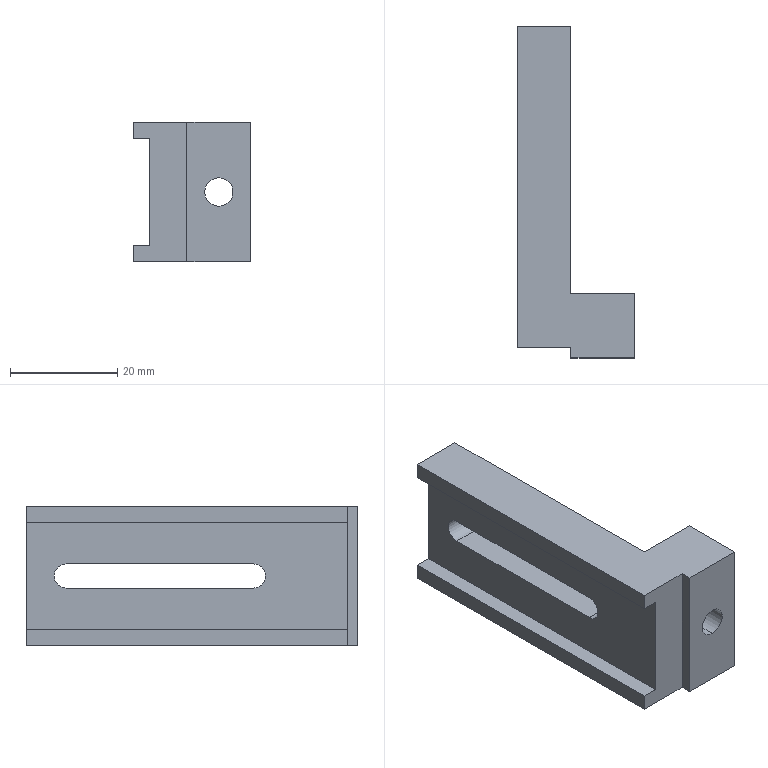Part | NX | features BREP 1 | 1 solid | 23 faces | box 21.97 x 62 x 26 mm | volume 13950 mm3 | plane 17 | cylinder 6 | commonest cylinder face diameters 4.5 x2 5.3 x2 10 x2
STEP:
#1=CARTESIAN_POINT('',(6.,-5.4,7.));
#2=VERTEX_POINT('',#1);
#3=CARTESIAN_POINT('',(6.,-5.4,17.));
#4=VERTEX_POINT('',#3);
#5=CARTESIAN_POINT('',(6.,-5.4,12.));
#6=DIRECTION('',(0.,1.,0.));
#7=DIRECTION('',(0.,0.,1.));
#8=AXIS2_PLACEMENT_3D('',#5,#6,#7);
#9=CIRCLE('',#8,5.);
#10=EDGE_CURVE('',#2,#4,#9,.T.);
#11=ORIENTED_EDGE('',*,*,#10,.F.);
#12=CARTESIAN_POINT('',(6.,0.,7.));
#13=VERTEX_POINT('',#12);
#14=CARTESIAN_POINT('',(6.,0.,7.));
#15=DIRECTION('',(0.,1.,0.));
#16=VECTOR('',#15,1000.);
#17=LINE('',#14,#16);
#18=EDGE_CURVE('',#13,#2,#17,.F.);
#19=ORIENTED_EDGE('',*,*,#18,.F.);
#20=CARTESIAN_POINT('',(6.,0.,17.));
#21=VERTEX_POINT('',#20);
#22=CARTESIAN_POINT('',(6.,0.,12.));
#23=DIRECTION('',(0.,1.,0.));
#24=DIRECTION('',(0.,0.,1.));
#25=AXIS2_PLACEMENT_3D('',#22,#23,#24);
#26=CIRCLE('',#25,5.);
#27=EDGE_CURVE('',#13,#21,#26,.T.);
#28=ORIENTED_EDGE('',*,*,#27,.T.);
#29=CARTESIAN_POINT('',(6.,0.,17.));
#30=DIRECTION('',(0.,1.,0.));
#31=VECTOR('',#30,1000.);
#32=LINE('',#29,#31);
#33=EDGE_CURVE('',#21,#4,#32,.F.);
#34=ORIENTED_EDGE('',*,*,#33,.T.);
#35=EDGE_LOOP('',(#11,#19,#28,#34));
#36=FACE_BOUND('',#35,.T.);
#37=CARTESIAN_POINT('',(6.,0.,12.));
#38=DIRECTION('',(0.,1.,0.));
#39=DIRECTION('',(0.,0.,1.));
#40=AXIS2_PLACEMENT_3D('',#37,#38,#39);
#41=CYLINDRICAL_SURFACE('',#40,5.);
#42=ADVANCED_FACE('',(#36),#41,.F.);
#43=CARTESIAN_POINT('',(6.,-12.,9.35));
#44=VERTEX_POINT('',#43);
#45=CARTESIAN_POINT('',(6.,-12.,14.65));
#46=VERTEX_POINT('',#45);
#47=CARTESIAN_POINT('',(6.,-12.,12.));
#48=DIRECTION('',(0.,1.,0.));
#49=DIRECTION('',(0.,0.,1.));
#50=AXIS2_PLACEMENT_3D('',#47,#48,#49);
#51=CIRCLE('',#50,2.65);
#52=EDGE_CURVE('',#44,#46,#51,.T.);
#53=ORIENTED_EDGE('',*,*,#52,.F.);
#54=CARTESIAN_POINT('',(6.,-5.4,9.35));
#55=VERTEX_POINT('',#54);
#56=CARTESIAN_POINT('',(6.,0.,9.35));
#57=DIRECTION('',(0.,1.,0.));
#58=VECTOR('',#57,1000.);
#59=LINE('',#56,#58);
#60=EDGE_CURVE('',#55,#44,#59,.F.);
#61=ORIENTED_EDGE('',*,*,#60,.F.);
#62=CARTESIAN_POINT('',(6.,-5.4,14.65));
#63=VERTEX_POINT('',#62);
#64=CARTESIAN_POINT('',(6.,-5.4,12.));
#65=DIRECTION('',(0.,1.,0.));
#66=DIRECTION('',(0.,0.,1.));
#67=AXIS2_PLACEMENT_3D('',#64,#65,#66);
#68=CIRCLE('',#67,2.65);
#69=EDGE_CURVE('',#55,#63,#68,.T.);
#70=ORIENTED_EDGE('',*,*,#69,.T.);
#71=CARTESIAN_POINT('',(6.,0.,14.65));
#72=DIRECTION('',(0.,1.,0.));
#73=VECTOR('',#72,1000.);
#74=LINE('',#71,#73);
#75=EDGE_CURVE('',#63,#46,#74,.F.);
#76=ORIENTED_EDGE('',*,*,#75,.T.);
#77=EDGE_LOOP('',(#53,#61,#70,#76));
#78=FACE_BOUND('',#77,.T.);
#79=CARTESIAN_POINT('',(6.,0.,12.));
#80=DIRECTION('',(0.,1.,0.));
#81=DIRECTION('',(0.,0.,1.));
#82=AXIS2_PLACEMENT_3D('',#79,#80,#81);
#83=CYLINDRICAL_SURFACE('',#82,2.65);
#84=ADVANCED_FACE('',(#78),#83,.F.);
#85=CARTESIAN_POINT('',(-10.,50.,25.));
#86=VERTEX_POINT('',#85);
#87=CARTESIAN_POINT('',(-10.,50.,22.));
#88=VERTEX_POINT('',#87);
#89=CARTESIAN_POINT('',(-10.,50.,24.));
#90=DIRECTION('',(0.,0.,-1.));
#91=VECTOR('',#90,1000.);
#92=LINE('',#89,#91);
#93=EDGE_CURVE('',#86,#88,#92,.T.);
#94=ORIENTED_EDGE('',*,*,#93,.T.);
#95=CARTESIAN_POINT('',(-10.,-10.,22.));
#96=VERTEX_POINT('',#95);
#97=CARTESIAN_POINT('',(-10.,0.,22.));
#98=DIRECTION('',(0.,-1.,0.));
#99=VECTOR('',#98,1000.);
#100=LINE('',#97,#99);
#101=EDGE_CURVE('',#88,#96,#100,.T.);
#102=ORIENTED_EDGE('',*,*,#101,.T.);
#103=CARTESIAN_POINT('',(-10.,-10.,25.));
#104=VERTEX_POINT('',#103);
#105=CARTESIAN_POINT('',(-10.,-10.,24.));
#106=DIRECTION('',(0.,0.,-1.));
#107=VECTOR('',#106,1000.);
#108=LINE('',#105,#107);
#109=EDGE_CURVE('',#104,#96,#108,.T.);
#110=ORIENTED_EDGE('',*,*,#109,.F.);
#111=CARTESIAN_POINT('',(-10.,0.,25.));
#112=DIRECTION('',(0.,-1.,0.));
#113=VECTOR('',#112,1000.);
#114=LINE('',#111,#113);
#115=EDGE_CURVE('',#86,#104,#114,.T.);
#116=ORIENTED_EDGE('',*,*,#115,.F.);
#117=EDGE_LOOP('',(#94,#102,#110,#116));
#118=FACE_BOUND('',#117,.T.);
#119=CARTESIAN_POINT('',(-10.,0.,24.));
#120=DIRECTION('',(1.,0.,0.));
#121=DIRECTION('',(0.,1.,0.));
#122=AXIS2_PLACEMENT_3D('',#119,#120,#121);
#123=PLANE('',#122);
#124=ADVANCED_FACE('',(#118),#123,.F.);
#125=ORIENTED_EDGE('',*,*,#109,.T.);
#126=CARTESIAN_POINT('',(-7.,-10.,22.));
#127=VERTEX_POINT('',#126);
#128=CARTESIAN_POINT('',(0.,-10.,22.));
#129=DIRECTION('',(1.,0.,0.));
#130=VECTOR('',#129,1000.);
#131=LINE('',#128,#130);
#132=EDGE_CURVE('',#96,#127,#131,.T.);
#133=ORIENTED_EDGE('',*,*,#132,.T.);
#134=CARTESIAN_POINT('',(-7.,-10.,2.));
#135=VERTEX_POINT('',#134);
#136=CARTESIAN_POINT('',(-7.,-10.,24.));
#137=DIRECTION('',(0.,0.,1.));
#138=VECTOR('',#137,1000.);
#139=LINE('',#136,#138);
#140=EDGE_CURVE('',#135,#127,#139,.T.);
#141=ORIENTED_EDGE('',*,*,#140,.F.);
#142=CARTESIAN_POINT('',(-10.,-10.,2.));
#143=VERTEX_POINT('',#142);
#144=CARTESIAN_POINT('',(0.,-10.,2.));
#145=DIRECTION('',(-1.,0.,0.));
#146=VECTOR('',#145,1000.);
#147=LINE('',#144,#146);
#148=EDGE_CURVE('',#135,#143,#147,.T.);
#149=ORIENTED_EDGE('',*,*,#148,.T.);
#150=CARTESIAN_POINT('',(-10.,-10.,-1.));
#151=VERTEX_POINT('',#150);
#152=CARTESIAN_POINT('',(-10.,-10.,24.));
#153=DIRECTION('',(0.,0.,-1.));
#154=VECTOR('',#153,1000.);
#155=LINE('',#152,#154);
#156=EDGE_CURVE('',#143,#151,#155,.T.);
#157=ORIENTED_EDGE('',*,*,#156,.T.);
#158=CARTESIAN_POINT('',(0.03,-10.,-1.));
#159=VERTEX_POINT('',#158);
#160=CARTESIAN_POINT('',(0.,-10.,-1.));
#161=DIRECTION('',(1.,0.,0.));
#162=VECTOR('',#161,1000.);
#163=LINE('',#160,#162);
#164=EDGE_CURVE('',#151,#159,#163,.T.);
#165=ORIENTED_EDGE('',*,*,#164,.T.);
#166=CARTESIAN_POINT('',(0.03,-10.,25.));
#167=VERTEX_POINT('',#166);
#168=CARTESIAN_POINT('',(0.03,-10.,0.));
#169=DIRECTION('',(0.,0.,-1.));
#170=VECTOR('',#169,1000.);
#171=LINE('',#168,#170);
#172=EDGE_CURVE('',#167,#159,#171,.T.);
#173=ORIENTED_EDGE('',*,*,#172,.F.);
#174=CARTESIAN_POINT('',(0.,-10.,25.));
#175=DIRECTION('',(1.,0.,0.));
#176=VECTOR('',#175,1000.);
#177=LINE('',#174,#176);
#178=EDGE_CURVE('',#104,#167,#177,.T.);
#179=ORIENTED_EDGE('',*,*,#178,.F.);
#180=EDGE_LOOP('',(#125,#133,#141,#149,#157,#165,#173,#179));
#181=FACE_BOUND('',#180,.T.);
#182=CARTESIAN_POINT('',(0.,-10.,24.));
#183=DIRECTION('',(0.,1.,0.));
#184=DIRECTION('',(1.,0.,0.));
#185=AXIS2_PLACEMENT_3D('',#182,#183,#184);
#186=PLANE('',#185);
#187=ADVANCED_FACE('',(#181),#186,.F.);
#188=CARTESIAN_POINT('',(11.97,0.,-1.));
#189=VERTEX_POINT('',#188);
#190=CARTESIAN_POINT('',(11.97,-12.,-1.));
#191=VERTEX_POINT('',#190);
#192=CARTESIAN_POINT('',(11.97,0.,-1.));
#193=DIRECTION('',(0.,-1.,0.));
#194=VECTOR('',#193,1000.);
#195=LINE('',#192,#194);
#196=EDGE_CURVE('',#189,#191,#195,.T.);
#197=ORIENTED_EDGE('',*,*,#196,.F.);
#198=CARTESIAN_POINT('',(11.97,0.,25.));
#199=VERTEX_POINT('',#198);
#200=CARTESIAN_POINT('',(11.97,0.,24.));
#201=DIRECTION('',(0.,0.,-1.));
#202=VECTOR('',#201,1000.);
#203=LINE('',#200,#202);
#204=EDGE_CURVE('',#199,#189,#203,.T.);
#205=ORIENTED_EDGE('',*,*,#204,.F.);
#206=CARTESIAN_POINT('',(11.97,-12.,25.));
#207=VERTEX_POINT('',#206);
#208=CARTESIAN_POINT('',(11.97,0.,25.));
#209=DIRECTION('',(0.,-1.,0.));
#210=VECTOR('',#209,1000.);
#211=LINE('',#208,#210);
#212=EDGE_CURVE('',#199,#207,#211,.T.);
#213=ORIENTED_EDGE('',*,*,#212,.T.);
#214=CARTESIAN_POINT('',(11.97,-12.,0.));
#215=DIRECTION('',(0.,0.,1.));
#216=VECTOR('',#215,1000.);
#217=LINE('',#214,#216);
#218=EDGE_CURVE('',#191,#207,#217,.T.);
#219=ORIENTED_EDGE('',*,*,#218,.F.);
#220=EDGE_LOOP('',(#197,#205,#213,#219));
#221=FACE_BOUND('',#220,.T.);
#222=CARTESIAN_POINT('',(11.97,0.,24.));
#223=DIRECTION('',(1.,0.,0.));
#224=DIRECTION('',(0.,1.,0.));
#225=AXIS2_PLACEMENT_3D('',#222,#223,#224);
#226=PLANE('',#225);
#227=ADVANCED_FACE('',(#221),#226,.T.);
#228=CARTESIAN_POINT('',(0.,0.,-1.));
#229=VERTEX_POINT('',#228);
#230=CARTESIAN_POINT('',(0.,0.,-1.));
#231=DIRECTION('',(1.,0.,0.));
#232=VECTOR('',#231,1000.);
#233=LINE('',#230,#232);
#234=EDGE_CURVE('',#229,#189,#233,.T.);
#235=ORIENTED_EDGE('',*,*,#234,.F.);
#236=CARTESIAN_POINT('',(0.,0.,25.));
#237=VERTEX_POINT('',#236);
#238=CARTESIAN_POINT('',(0.,0.,24.));
#239=DIRECTION('',(0.,0.,-1.));
#240=VECTOR('',#239,1000.);
#241=LINE('',#238,#240);
#242=EDGE_CURVE('',#237,#229,#241,.T.);
#243=ORIENTED_EDGE('',*,*,#242,.F.);
#244=CARTESIAN_POINT('',(0.,0.,25.));
#245=DIRECTION('',(1.,0.,0.));
#246=VECTOR('',#245,1000.);
#247=LINE('',#244,#246);
#248=EDGE_CURVE('',#237,#199,#247,.T.);
#249=ORIENTED_EDGE('',*,*,#248,.T.);
#250=ORIENTED_EDGE('',*,*,#204,.T.);
#251=EDGE_LOOP('',(#235,#243,#249,#250));
#252=FACE_BOUND('',#251,.T.);
#253=CARTESIAN_POINT('',(6.,0.,12.));
#254=DIRECTION('',(0.,1.,0.));
#255=DIRECTION('',(0.,0.,1.));
#256=AXIS2_PLACEMENT_3D('',#253,#254,#255);
#257=CIRCLE('',#256,5.);
#258=EDGE_CURVE('',#21,#13,#257,.T.);
#259=ORIENTED_EDGE('',*,*,#258,.F.);
#260=ORIENTED_EDGE('',*,*,#27,.F.);
#261=EDGE_LOOP('',(#259,#260));
#262=FACE_BOUND('',#261,.T.);
#263=CARTESIAN_POINT('',(0.,0.,24.));
#264=DIRECTION('',(0.,1.,0.));
#265=DIRECTION('',(1.,0.,0.));
#266=AXIS2_PLACEMENT_3D('',#263,#264,#265);
#267=PLANE('',#266);
#268=ADVANCED_FACE('',(#252,#262),#267,.T.);
#269=CARTESIAN_POINT('',(0.,50.,-1.));
#270=VERTEX_POINT('',#269);
#271=CARTESIAN_POINT('',(0.,0.,-1.));
#272=DIRECTION('',(0.,-1.,0.));
#273=VECTOR('',#272,1000.);
#274=LINE('',#271,#273);
#275=EDGE_CURVE('',#270,#229,#274,.T.);
#276=ORIENTED_EDGE('',*,*,#275,.F.);
#277=CARTESIAN_POINT('',(0.,50.,25.));
#278=VERTEX_POINT('',#277);
#279=CARTESIAN_POINT('',(0.,50.,24.));
#280=DIRECTION('',(0.,0.,-1.));
#281=VECTOR('',#280,1000.);
#282=LINE('',#279,#281);
#283=EDGE_CURVE('',#278,#270,#282,.T.);
#284=ORIENTED_EDGE('',*,*,#283,.F.);
#285=CARTESIAN_POINT('',(0.,0.,25.));
#286=DIRECTION('',(0.,-1.,0.));
#287=VECTOR('',#286,1000.);
#288=LINE('',#285,#287);
#289=EDGE_CURVE('',#278,#237,#288,.T.);
#290=ORIENTED_EDGE('',*,*,#289,.T.);
#291=ORIENTED_EDGE('',*,*,#242,.T.);
#292=EDGE_LOOP('',(#276,#284,#290,#291));
#293=FACE_BOUND('',#292,.T.);
#294=CARTESIAN_POINT('',(0.,7.5,14.25));
#295=VERTEX_POINT('',#294);
#296=CARTESIAN_POINT('',(0.,7.5,9.75));
#297=VERTEX_POINT('',#296);
#298=CARTESIAN_POINT('',(0.,7.5,12.));
#299=DIRECTION('',(1.,0.,0.));
#300=DIRECTION('',(0.,0.,-1.));
#301=AXIS2_PLACEMENT_3D('',#298,#299,#300);
#302=CIRCLE('',#301,2.25);
#303=EDGE_CURVE('',#295,#297,#302,.T.);
#304=ORIENTED_EDGE('',*,*,#303,.F.);
#305=CARTESIAN_POINT('',(0.,42.5,14.25));
#306=VERTEX_POINT('',#305);
#307=CARTESIAN_POINT('',(0.,7.5,14.25));
#308=DIRECTION('',(0.,-1.,0.));
#309=VECTOR('',#308,1000.);
#310=LINE('',#307,#309);
#311=EDGE_CURVE('',#306,#295,#310,.T.);
#312=ORIENTED_EDGE('',*,*,#311,.F.);
#313=CARTESIAN_POINT('',(0.,42.5,9.75));
#314=VERTEX_POINT('',#313);
#315=CARTESIAN_POINT('',(0.,42.5,12.));
#316=DIRECTION('',(1.,0.,0.));
#317=DIRECTION('',(0.,0.,-1.));
#318=AXIS2_PLACEMENT_3D('',#315,#316,#317);
#319=CIRCLE('',#318,2.25);
#320=EDGE_CURVE('',#314,#306,#319,.T.);
#321=ORIENTED_EDGE('',*,*,#320,.F.);
#322=CARTESIAN_POINT('',(0.,7.5,9.75));
#323=DIRECTION('',(0.,1.,0.));
#324=VECTOR('',#323,1000.);
#325=LINE('',#322,#324);
#326=EDGE_CURVE('',#297,#314,#325,.T.);
#327=ORIENTED_EDGE('',*,*,#326,.F.);
#328=EDGE_LOOP('',(#304,#312,#321,#327));
#329=FACE_BOUND('',#328,.T.);
#330=CARTESIAN_POINT('',(0.,0.,24.));
#331=DIRECTION('',(1.,0.,0.));
#332=DIRECTION('',(0.,1.,0.));
#333=AXIS2_PLACEMENT_3D('',#330,#331,#332);
#334=PLANE('',#333);
#335=ADVANCED_FACE('',(#293,#329),#334,.T.);
#336=CARTESIAN_POINT('',(-7.,50.,22.));
#337=VERTEX_POINT('',#336);
#338=CARTESIAN_POINT('',(-10.,50.,22.));
#339=DIRECTION('',(1.,0.,0.));
#340=VECTOR('',#339,1000.);
#341=LINE('',#338,#340);
#342=EDGE_CURVE('',#88,#337,#341,.T.);
#343=ORIENTED_EDGE('',*,*,#342,.F.);
#344=ORIENTED_EDGE('',*,*,#93,.F.);
#345=CARTESIAN_POINT('',(-10.,50.,25.));
#346=DIRECTION('',(1.,0.,0.));
#347=VECTOR('',#346,1000.);
#348=LINE('',#345,#347);
#349=EDGE_CURVE('',#86,#278,#348,.T.);
#350=ORIENTED_EDGE('',*,*,#349,.T.);
#351=ORIENTED_EDGE('',*,*,#283,.T.);
#352=CARTESIAN_POINT('',(-10.,50.,-1.));
#353=VERTEX_POINT('',#352);
#354=CARTESIAN_POINT('',(-10.,50.,-1.));
#355=DIRECTION('',(1.,0.,0.));
#356=VECTOR('',#355,1000.);
#357=LINE('',#354,#356);
#358=EDGE_CURVE('',#353,#270,#357,.T.);
#359=ORIENTED_EDGE('',*,*,#358,.F.);
#360=CARTESIAN_POINT('',(-10.,50.,2.));
#361=VERTEX_POINT('',#360);
#362=CARTESIAN_POINT('',(-10.,50.,24.));
#363=DIRECTION('',(0.,0.,-1.));
#364=VECTOR('',#363,1000.);
#365=LINE('',#362,#364);
#366=EDGE_CURVE('',#361,#353,#365,.T.);
#367=ORIENTED_EDGE('',*,*,#366,.F.);
#368=CARTESIAN_POINT('',(-7.,50.,2.));
#369=VERTEX_POINT('',#368);
#370=CARTESIAN_POINT('',(-10.,50.,2.));
#371=DIRECTION('',(-1.,0.,0.));
#372=VECTOR('',#371,1000.);
#373=LINE('',#370,#372);
#374=EDGE_CURVE('',#369,#361,#373,.T.);
#375=ORIENTED_EDGE('',*,*,#374,.F.);
#376=CARTESIAN_POINT('',(-7.,50.,24.));
#377=DIRECTION('',(0.,0.,1.));
#378=VECTOR('',#377,1000.);
#379=LINE('',#376,#378);
#380=EDGE_CURVE('',#369,#337,#379,.T.);
#381=ORIENTED_EDGE('',*,*,#380,.T.);
#382=EDGE_LOOP('',(#343,#344,#350,#351,#359,#367,#375,#381));
#383=FACE_BOUND('',#382,.T.);
#384=CARTESIAN_POINT('',(-10.,50.,24.));
#385=DIRECTION('',(0.,1.,0.));
#386=DIRECTION('',(1.,0.,0.));
#387=AXIS2_PLACEMENT_3D('',#384,#385,#386);
#388=PLANE('',#387);
#389=ADVANCED_FACE('',(#383),#388,.T.);
#390=ORIENTED_EDGE('',*,*,#156,.F.);
#391=CARTESIAN_POINT('',(-10.,0.,2.));
#392=DIRECTION('',(0.,1.,0.));
#393=VECTOR('',#392,1000.);
#394=LINE('',#391,#393);
#395=EDGE_CURVE('',#143,#361,#394,.T.);
#396=ORIENTED_EDGE('',*,*,#395,.T.);
#397=ORIENTED_EDGE('',*,*,#366,.T.);
#398=CARTESIAN_POINT('',(-10.,0.,-1.));
#399=DIRECTION('',(0.,-1.,0.));
#400=VECTOR('',#399,1000.);
#401=LINE('',#398,#400);
#402=EDGE_CURVE('',#353,#151,#401,.T.);
#403=ORIENTED_EDGE('',*,*,#402,.T.);
#404=EDGE_LOOP('',(#390,#396,#397,#403));
#405=FACE_BOUND('',#404,.T.);
#406=CARTESIAN_POINT('',(-10.,0.,24.));
#407=DIRECTION('',(1.,0.,0.));
#408=DIRECTION('',(0.,1.,0.));
#409=AXIS2_PLACEMENT_3D('',#406,#407,#408);
#410=PLANE('',#409);
#411=ADVANCED_FACE('',(#405),#410,.F.);
#412=ORIENTED_EDGE('',*,*,#178,.T.);
#413=CARTESIAN_POINT('',(0.03,-12.,25.));
#414=VERTEX_POINT('',#413);
#415=CARTESIAN_POINT('',(0.03,-12.,25.));
#416=DIRECTION('',(0.,1.,0.));
#417=VECTOR('',#416,1000.);
#418=LINE('',#415,#417);
#419=EDGE_CURVE('',#414,#167,#418,.T.);
#420=ORIENTED_EDGE('',*,*,#419,.F.);
#421=CARTESIAN_POINT('',(0.,-12.,25.));
#422=DIRECTION('',(-1.,0.,0.));
#423=VECTOR('',#422,1000.);
#424=LINE('',#421,#423);
#425=EDGE_CURVE('',#207,#414,#424,.T.);
#426=ORIENTED_EDGE('',*,*,#425,.F.);
#427=ORIENTED_EDGE('',*,*,#212,.F.);
#428=ORIENTED_EDGE('',*,*,#248,.F.);
#429=ORIENTED_EDGE('',*,*,#289,.F.);
#430=ORIENTED_EDGE('',*,*,#349,.F.);
#431=ORIENTED_EDGE('',*,*,#115,.T.);
#432=EDGE_LOOP('',(#412,#420,#426,#427,#428,#429,#430,#431));
#433=FACE_BOUND('',#432,.T.);
#434=CARTESIAN_POINT('',(0.,0.,25.));
#435=DIRECTION('',(0.,0.,-1.));
#436=DIRECTION('',(0.,-1.,0.));
#437=AXIS2_PLACEMENT_3D('',#434,#435,#436);
#438=PLANE('',#437);
#439=ADVANCED_FACE('',(#433),#438,.F.);
#440=ORIENTED_EDGE('',*,*,#164,.F.);
#441=ORIENTED_EDGE('',*,*,#402,.F.);
#442=ORIENTED_EDGE('',*,*,#358,.T.);
#443=ORIENTED_EDGE('',*,*,#275,.T.);
#444=ORIENTED_EDGE('',*,*,#234,.T.);
#445=ORIENTED_EDGE('',*,*,#196,.T.);
#446=CARTESIAN_POINT('',(0.03,-12.,-1.));
#447=VERTEX_POINT('',#446);
#448=CARTESIAN_POINT('',(0.,-12.,-1.));
#449=DIRECTION('',(1.,0.,0.));
#450=VECTOR('',#449,1000.);
#451=LINE('',#448,#450);
#452=EDGE_CURVE('',#447,#191,#451,.T.);
#453=ORIENTED_EDGE('',*,*,#452,.F.);
#454=CARTESIAN_POINT('',(0.03,-12.,-1.));
#455=DIRECTION('',(0.,1.,0.));
#456=VECTOR('',#455,1000.);
#457=LINE('',#454,#456);
#458=EDGE_CURVE('',#447,#159,#457,.T.);
#459=ORIENTED_EDGE('',*,*,#458,.T.);
#460=EDGE_LOOP('',(#440,#441,#442,#443,#444,#445,#453,#459));
#461=FACE_BOUND('',#460,.T.);
#462=CARTESIAN_POINT('',(0.,0.,-1.));
#463=DIRECTION('',(0.,0.,-1.));
#464=DIRECTION('',(0.,-1.,0.));
#465=AXIS2_PLACEMENT_3D('',#462,#463,#464);
#466=PLANE('',#465);
#467=ADVANCED_FACE('',(#461),#466,.T.);
#468=ORIENTED_EDGE('',*,*,#172,.T.);
#469=ORIENTED_EDGE('',*,*,#458,.F.);
#470=CARTESIAN_POINT('',(0.03,-12.,0.));
#471=DIRECTION('',(0.,0.,-1.));
#472=VECTOR('',#471,1000.);
#473=LINE('',#470,#472);
#474=EDGE_CURVE('',#414,#447,#473,.T.);
#475=ORIENTED_EDGE('',*,*,#474,.F.);
#476=ORIENTED_EDGE('',*,*,#419,.T.);
#477=EDGE_LOOP('',(#468,#469,#475,#476));
#478=FACE_BOUND('',#477,.T.);
#479=CARTESIAN_POINT('',(0.03,-12.,0.));
#480=DIRECTION('',(1.,0.,0.));
#481=DIRECTION('',(0.,1.,0.));
#482=AXIS2_PLACEMENT_3D('',#479,#480,#481);
#483=PLANE('',#482);
#484=ADVANCED_FACE('',(#478),#483,.F.);
#485=ORIENTED_EDGE('',*,*,#218,.T.);
#486=ORIENTED_EDGE('',*,*,#425,.T.);
#487=ORIENTED_EDGE('',*,*,#474,.T.);
#488=ORIENTED_EDGE('',*,*,#452,.T.);
#489=EDGE_LOOP('',(#485,#486,#487,#488));
#490=FACE_BOUND('',#489,.T.);
#491=CARTESIAN_POINT('',(6.,-12.,12.));
#492=DIRECTION('',(0.,1.,0.));
#493=DIRECTION('',(0.,0.,1.));
#494=AXIS2_PLACEMENT_3D('',#491,#492,#493);
#495=CIRCLE('',#494,2.65);
#496=EDGE_CURVE('',#46,#44,#495,.T.);
#497=ORIENTED_EDGE('',*,*,#496,.T.);
#498=ORIENTED_EDGE('',*,*,#52,.T.);
#499=EDGE_LOOP('',(#497,#498));
#500=FACE_BOUND('',#499,.T.);
#501=CARTESIAN_POINT('',(0.,-12.,0.));
#502=DIRECTION('',(0.,1.,0.));
#503=DIRECTION('',(1.,0.,0.));
#504=AXIS2_PLACEMENT_3D('',#501,#502,#503);
#505=PLANE('',#504);
#506=ADVANCED_FACE('',(#490,#500),#505,.F.);
#507=ORIENTED_EDGE('',*,*,#60,.T.);
#508=ORIENTED_EDGE('',*,*,#496,.F.);
#509=ORIENTED_EDGE('',*,*,#75,.F.);
#510=CARTESIAN_POINT('',(6.,-5.4,12.));
#511=DIRECTION('',(0.,1.,0.));
#512=DIRECTION('',(0.,0.,1.));
#513=AXIS2_PLACEMENT_3D('',#510,#511,#512);
#514=CIRCLE('',#513,2.65);
#515=EDGE_CURVE('',#63,#55,#514,.T.);
#516=ORIENTED_EDGE('',*,*,#515,.T.);
#517=EDGE_LOOP('',(#507,#508,#509,#516));
#518=FACE_BOUND('',#517,.T.);
#519=CARTESIAN_POINT('',(6.,0.,12.));
#520=DIRECTION('',(0.,1.,0.));
#521=DIRECTION('',(0.,0.,1.));
#522=AXIS2_PLACEMENT_3D('',#519,#520,#521);
#523=CYLINDRICAL_SURFACE('',#522,2.65);
#524=ADVANCED_FACE('',(#518),#523,.F.);
#525=CARTESIAN_POINT('',(6.,-5.4,12.));
#526=DIRECTION('',(0.,1.,0.));
#527=DIRECTION('',(0.,0.,1.));
#528=AXIS2_PLACEMENT_3D('',#525,#526,#527);
#529=CIRCLE('',#528,5.);
#530=EDGE_CURVE('',#4,#2,#529,.T.);
#531=ORIENTED_EDGE('',*,*,#530,.T.);
#532=ORIENTED_EDGE('',*,*,#10,.T.);
#533=EDGE_LOOP('',(#531,#532));
#534=FACE_BOUND('',#533,.T.);
#535=ORIENTED_EDGE('',*,*,#515,.F.);
#536=ORIENTED_EDGE('',*,*,#69,.F.);
#537=EDGE_LOOP('',(#535,#536));
#538=FACE_BOUND('',#537,.T.);
#539=CARTESIAN_POINT('',(8.65,-5.4,12.));
#540=DIRECTION('',(0.,-1.,0.));
#541=DIRECTION('',(0.,0.,-1.));
#542=AXIS2_PLACEMENT_3D('',#539,#540,#541);
#543=PLANE('',#542);
#544=ADVANCED_FACE('',(#534,#538),#543,.F.);
#545=ORIENTED_EDGE('',*,*,#18,.T.);
#546=ORIENTED_EDGE('',*,*,#530,.F.);
#547=ORIENTED_EDGE('',*,*,#33,.F.);
#548=ORIENTED_EDGE('',*,*,#258,.T.);
#549=EDGE_LOOP('',(#545,#546,#547,#548));
#550=FACE_BOUND('',#549,.T.);
#551=CARTESIAN_POINT('',(6.,0.,12.));
#552=DIRECTION('',(0.,1.,0.));
#553=DIRECTION('',(0.,0.,1.));
#554=AXIS2_PLACEMENT_3D('',#551,#552,#553);
#555=CYLINDRICAL_SURFACE('',#554,5.);
#556=ADVANCED_FACE('',(#550),#555,.F.);
#557=ORIENTED_EDGE('',*,*,#140,.T.);
#558=CARTESIAN_POINT('',(-7.,110.578,22.));
#559=DIRECTION('',(0.,1.,0.));
#560=VECTOR('',#559,1000.);
#561=LINE('',#558,#560);
#562=EDGE_CURVE('',#127,#337,#561,.T.);
#563=ORIENTED_EDGE('',*,*,#562,.T.);
#564=ORIENTED_EDGE('',*,*,#380,.F.);
#565=CARTESIAN_POINT('',(-7.,110.578,2.));
#566=DIRECTION('',(0.,-1.,0.));
#567=VECTOR('',#566,1000.);
#568=LINE('',#565,#567);
#569=EDGE_CURVE('',#369,#135,#568,.T.);
#570=ORIENTED_EDGE('',*,*,#569,.T.);
#571=EDGE_LOOP('',(#557,#563,#564,#570));
#572=FACE_BOUND('',#571,.T.);
#573=CARTESIAN_POINT('',(-7.,7.5,9.75));
#574=VERTEX_POINT('',#573);
#575=CARTESIAN_POINT('',(-7.,7.5,14.25));
#576=VERTEX_POINT('',#575);
#577=CARTESIAN_POINT('',(-7.,7.5,12.));
#578=DIRECTION('',(-1.,0.,0.));
#579=DIRECTION('',(0.,0.,1.));
#580=AXIS2_PLACEMENT_3D('',#577,#578,#579);
#581=CIRCLE('',#580,2.25);
#582=EDGE_CURVE('',#574,#576,#581,.T.);
#583=ORIENTED_EDGE('',*,*,#582,.F.);
#584=CARTESIAN_POINT('',(-7.,42.5,9.75));
#585=VERTEX_POINT('',#584);
#586=CARTESIAN_POINT('',(-7.,0.,9.75));
#587=DIRECTION('',(0.,-1.,0.));
#588=VECTOR('',#587,1000.);
#589=LINE('',#586,#588);
#590=EDGE_CURVE('',#585,#574,#589,.T.);
#591=ORIENTED_EDGE('',*,*,#590,.F.);
#592=CARTESIAN_POINT('',(-7.,42.5,14.25));
#593=VERTEX_POINT('',#592);
#594=CARTESIAN_POINT('',(-7.,42.5,12.));
#595=DIRECTION('',(-1.,0.,0.));
#596=DIRECTION('',(0.,0.,1.));
#597=AXIS2_PLACEMENT_3D('',#594,#595,#596);
#598=CIRCLE('',#597,2.25);
#599=EDGE_CURVE('',#593,#585,#598,.T.);
#600=ORIENTED_EDGE('',*,*,#599,.F.);
#601=CARTESIAN_POINT('',(-7.,0.,14.25));
#602=DIRECTION('',(0.,1.,0.));
#603=VECTOR('',#602,1000.);
#604=LINE('',#601,#603);
#605=EDGE_CURVE('',#576,#593,#604,.T.);
#606=ORIENTED_EDGE('',*,*,#605,.F.);
#607=EDGE_LOOP('',(#583,#591,#600,#606));
#608=FACE_BOUND('',#607,.T.);
#609=CARTESIAN_POINT('',(-7.,0.,0.));
#610=DIRECTION('',(-1.,0.,0.));
#611=DIRECTION('',(0.,0.,1.));
#612=AXIS2_PLACEMENT_3D('',#609,#610,#611);
#613=PLANE('',#612);
#614=ADVANCED_FACE('',(#572,#608),#613,.T.);
#615=ORIENTED_EDGE('',*,*,#101,.F.);
#616=ORIENTED_EDGE('',*,*,#342,.T.);
#617=ORIENTED_EDGE('',*,*,#562,.F.);
#618=ORIENTED_EDGE('',*,*,#132,.F.);
#619=EDGE_LOOP('',(#615,#616,#617,#618));
#620=FACE_BOUND('',#619,.T.);
#621=CARTESIAN_POINT('',(-7.,110.578,22.));
#622=DIRECTION('',(0.,0.,1.));
#623=DIRECTION('',(0.,-1.,0.));
#624=AXIS2_PLACEMENT_3D('',#621,#622,#623);
#625=PLANE('',#624);
#626=ADVANCED_FACE('',(#620),#625,.F.);
#627=ORIENTED_EDGE('',*,*,#569,.F.);
#628=ORIENTED_EDGE('',*,*,#374,.T.);
#629=ORIENTED_EDGE('',*,*,#395,.F.);
#630=ORIENTED_EDGE('',*,*,#148,.F.);
#631=EDGE_LOOP('',(#627,#628,#629,#630));
#632=FACE_BOUND('',#631,.T.);
#633=CARTESIAN_POINT('',(-7.,110.578,2.));
#634=DIRECTION('',(0.,0.,-1.));
#635=DIRECTION('',(0.,-1.,0.));
#636=AXIS2_PLACEMENT_3D('',#633,#634,#635);
#637=PLANE('',#636);
#638=ADVANCED_FACE('',(#632),#637,.F.);
#639=ORIENTED_EDGE('',*,*,#582,.T.);
#640=CARTESIAN_POINT('',(-10.,7.5,14.25));
#641=DIRECTION('',(1.,0.,0.));
#642=VECTOR('',#641,1000.);
#643=LINE('',#640,#642);
#644=EDGE_CURVE('',#576,#295,#643,.T.);
#645=ORIENTED_EDGE('',*,*,#644,.T.);
#646=ORIENTED_EDGE('',*,*,#303,.T.);
#647=CARTESIAN_POINT('',(-10.,7.5,9.75));
#648=DIRECTION('',(1.,0.,0.));
#649=VECTOR('',#648,1000.);
#650=LINE('',#647,#649);
#651=EDGE_CURVE('',#574,#297,#650,.T.);
#652=ORIENTED_EDGE('',*,*,#651,.F.);
#653=EDGE_LOOP('',(#639,#645,#646,#652));
#654=FACE_BOUND('',#653,.T.);
#655=CARTESIAN_POINT('',(-10.,7.5,12.));
#656=DIRECTION('',(1.,0.,0.));
#657=DIRECTION('',(0.,0.,-1.));
#658=AXIS2_PLACEMENT_3D('',#655,#656,#657);
#659=CYLINDRICAL_SURFACE('',#658,2.25);
#660=ADVANCED_FACE('',(#654),#659,.F.);
#661=ORIENTED_EDGE('',*,*,#605,.T.);
#662=CARTESIAN_POINT('',(-10.,42.5,14.25));
#663=DIRECTION('',(1.,0.,0.));
#664=VECTOR('',#663,1000.);
#665=LINE('',#662,#664);
#666=EDGE_CURVE('',#593,#306,#665,.T.);
#667=ORIENTED_EDGE('',*,*,#666,.T.);
#668=ORIENTED_EDGE('',*,*,#311,.T.);
#669=ORIENTED_EDGE('',*,*,#644,.F.);
#670=EDGE_LOOP('',(#661,#667,#668,#669));
#671=FACE_BOUND('',#670,.T.);
#672=CARTESIAN_POINT('',(-10.,7.5,14.25));
#673=DIRECTION('',(0.,0.,1.));
#674=DIRECTION('',(0.,-1.,0.));
#675=AXIS2_PLACEMENT_3D('',#672,#673,#674);
#676=PLANE('',#675);
#677=ADVANCED_FACE('',(#671),#676,.F.);
#678=ORIENTED_EDGE('',*,*,#599,.T.);
#679=CARTESIAN_POINT('',(-10.,42.5,9.75));
#680=DIRECTION('',(1.,0.,0.));
#681=VECTOR('',#680,1000.);
#682=LINE('',#679,#681);
#683=EDGE_CURVE('',#585,#314,#682,.T.);
#684=ORIENTED_EDGE('',*,*,#683,.T.);
#685=ORIENTED_EDGE('',*,*,#320,.T.);
#686=ORIENTED_EDGE('',*,*,#666,.F.);
#687=EDGE_LOOP('',(#678,#684,#685,#686));
#688=FACE_BOUND('',#687,.T.);
#689=CARTESIAN_POINT('',(-10.,42.5,12.));
#690=DIRECTION('',(1.,0.,0.));
#691=DIRECTION('',(0.,0.,-1.));
#692=AXIS2_PLACEMENT_3D('',#689,#690,#691);
#693=CYLINDRICAL_SURFACE('',#692,2.25);
#694=ADVANCED_FACE('',(#688),#693,.F.);
#695=ORIENTED_EDGE('',*,*,#590,.T.);
#696=ORIENTED_EDGE('',*,*,#651,.T.);
#697=ORIENTED_EDGE('',*,*,#326,.T.);
#698=ORIENTED_EDGE('',*,*,#683,.F.);
#699=EDGE_LOOP('',(#695,#696,#697,#698));
#700=FACE_BOUND('',#699,.T.);
#701=CARTESIAN_POINT('',(-10.,7.5,9.75));
#702=DIRECTION('',(0.,0.,-1.));
#703=DIRECTION('',(-1.,0.,0.));
#704=AXIS2_PLACEMENT_3D('',#701,#702,#703);
#705=PLANE('',#704);
#706=ADVANCED_FACE('',(#700),#705,.F.);
#707=CLOSED_SHELL('',(#42,#84,#124,#187,#227,#268,#335,#389,#411,#439,#467,#484,#506,#524,#544,#556,#614,#626,#638,#660,#677,#694,#706));
#708=MANIFOLD_SOLID_BREP('',#707);
#709=(LENGTH_UNIT()NAMED_UNIT(*)SI_UNIT(.MILLI.,.METRE.));
#710=UNCERTAINTY_MEASURE_WITH_UNIT(LENGTH_MEASURE(0.00001),#709,'','');
#711=(NAMED_UNIT(*)PLANE_ANGLE_UNIT()SI_UNIT($,.RADIAN.));
#712=(NAMED_UNIT(*)SI_UNIT($,.STERADIAN.)SOLID_ANGLE_UNIT());
#713=(GEOMETRIC_REPRESENTATION_CONTEXT(3)GLOBAL_UNCERTAINTY_ASSIGNED_CONTEXT((#710))GLOBAL_UNIT_ASSIGNED_CONTEXT((#709,#711,#712))REPRESENTATION_CONTEXT('',''));
#714=ADVANCED_BREP_SHAPE_REPRESENTATION('',(#708),#713);